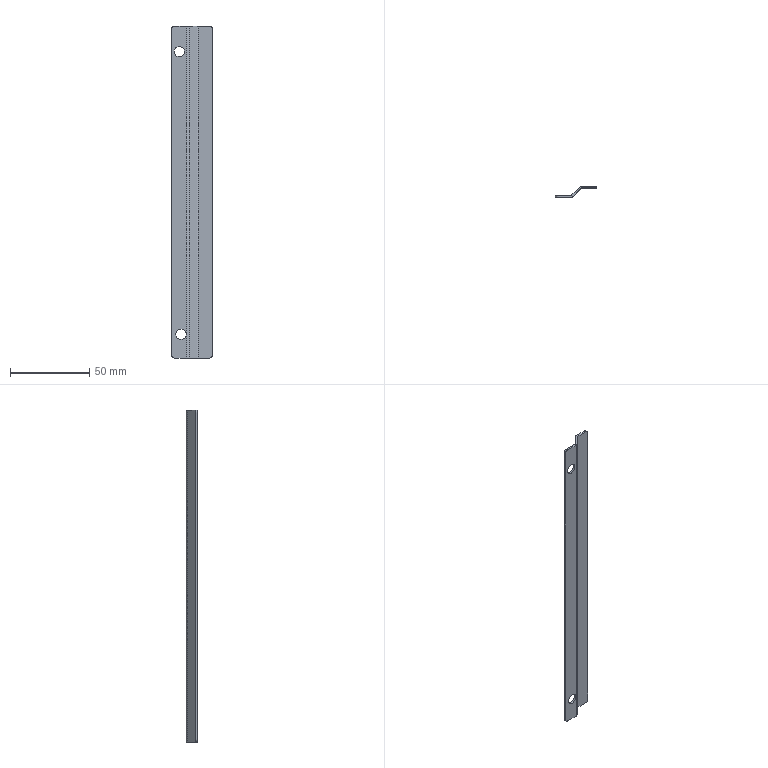Part | SolidWorks | features BreakCorner 1, FlatPattern 1, ICE 1, SMBaseFlange 1, SheetMetal 1 | 1 solid | 30 faces | box 26 x 7.2 x 210 mm | volume 7055 mm3 | plane 18 | cylinder 12 | commonest cylinder face diameters 4 x4 6.5 x4 2.4 x2 4.8 x2
STEP:
#1=CARTESIAN_POINT('',(6.,-1.2,11.75));
#2=VERTEX_POINT('',#1);
#3=CARTESIAN_POINT('',(6.,-1.2,18.25));
#4=VERTEX_POINT('',#3);
#5=CARTESIAN_POINT('',(6.,-1.2,15.));
#6=DIRECTION('',(0.,1.,0.));
#7=DIRECTION('',(0.,0.,1.));
#8=AXIS2_PLACEMENT_3D('',#5,#6,#7);
#9=CIRCLE('',#8,3.25);
#10=EDGE_CURVE('',#2,#4,#9,.T.);
#11=ORIENTED_EDGE('',*,*,#10,.F.);
#12=CARTESIAN_POINT('',(6.,0.,11.75));
#13=VERTEX_POINT('',#12);
#14=CARTESIAN_POINT('',(6.,-10.,11.75));
#15=DIRECTION('',(0.,1.,0.));
#16=VECTOR('',#15,1000.);
#17=LINE('',#14,#16);
#18=EDGE_CURVE('',#2,#13,#17,.T.);
#19=ORIENTED_EDGE('',*,*,#18,.T.);
#20=CARTESIAN_POINT('',(6.,0.,18.25));
#21=VERTEX_POINT('',#20);
#22=CARTESIAN_POINT('',(6.,0.,15.));
#23=DIRECTION('',(0.,1.,0.));
#24=DIRECTION('',(0.,0.,1.));
#25=AXIS2_PLACEMENT_3D('',#22,#23,#24);
#26=CIRCLE('',#25,3.25);
#27=EDGE_CURVE('',#13,#21,#26,.T.);
#28=ORIENTED_EDGE('',*,*,#27,.T.);
#29=CARTESIAN_POINT('',(6.,-10.,18.25));
#30=DIRECTION('',(0.,1.,0.));
#31=VECTOR('',#30,1000.);
#32=LINE('',#29,#31);
#33=EDGE_CURVE('',#4,#21,#32,.T.);
#34=ORIENTED_EDGE('',*,*,#33,.F.);
#35=EDGE_LOOP('',(#11,#19,#28,#34));
#36=FACE_OUTER_BOUND('',#35,.T.);
#37=CARTESIAN_POINT('',(6.,-10.,15.));
#38=DIRECTION('',(0.,1.,0.));
#39=DIRECTION('',(0.,0.,1.));
#40=AXIS2_PLACEMENT_3D('',#37,#38,#39);
#41=CYLINDRICAL_SURFACE('',#40,3.25);
#42=ADVANCED_FACE('',(#36),#41,.F.);
#43=CARTESIAN_POINT('',(5.,-1.2,190.542));
#44=VERTEX_POINT('',#43);
#45=CARTESIAN_POINT('',(5.,-1.2,197.042));
#46=VERTEX_POINT('',#45);
#47=CARTESIAN_POINT('',(5.,-1.2,193.792));
#48=DIRECTION('',(0.,1.,0.));
#49=DIRECTION('',(0.,0.,1.));
#50=AXIS2_PLACEMENT_3D('',#47,#48,#49);
#51=CIRCLE('',#50,3.25);
#52=EDGE_CURVE('',#44,#46,#51,.T.);
#53=ORIENTED_EDGE('',*,*,#52,.F.);
#54=CARTESIAN_POINT('',(5.,0.,190.542));
#55=VERTEX_POINT('',#54);
#56=CARTESIAN_POINT('',(5.,-10.,190.542));
#57=DIRECTION('',(0.,1.,0.));
#58=VECTOR('',#57,1000.);
#59=LINE('',#56,#58);
#60=EDGE_CURVE('',#44,#55,#59,.T.);
#61=ORIENTED_EDGE('',*,*,#60,.T.);
#62=CARTESIAN_POINT('',(5.,0.,197.042));
#63=VERTEX_POINT('',#62);
#64=CARTESIAN_POINT('',(5.,0.,193.792));
#65=DIRECTION('',(0.,1.,0.));
#66=DIRECTION('',(0.,0.,1.));
#67=AXIS2_PLACEMENT_3D('',#64,#65,#66);
#68=CIRCLE('',#67,3.25);
#69=EDGE_CURVE('',#55,#63,#68,.T.);
#70=ORIENTED_EDGE('',*,*,#69,.T.);
#71=CARTESIAN_POINT('',(5.,-10.,197.042));
#72=DIRECTION('',(0.,1.,0.));
#73=VECTOR('',#72,1000.);
#74=LINE('',#71,#73);
#75=EDGE_CURVE('',#46,#63,#74,.T.);
#76=ORIENTED_EDGE('',*,*,#75,.F.);
#77=EDGE_LOOP('',(#53,#61,#70,#76));
#78=FACE_OUTER_BOUND('',#77,.T.);
#79=CARTESIAN_POINT('',(5.,-10.,193.792));
#80=DIRECTION('',(0.,1.,0.));
#81=DIRECTION('',(0.,0.,1.));
#82=AXIS2_PLACEMENT_3D('',#79,#80,#81);
#83=CYLINDRICAL_SURFACE('',#82,3.25);
#84=ADVANCED_FACE('',(#78),#83,.F.);
#85=CARTESIAN_POINT('',(10.351,0.3515,210.));
#86=VERTEX_POINT('',#85);
#87=CARTESIAN_POINT('',(11.2,-0.4971,210.));
#88=VERTEX_POINT('',#87);
#89=CARTESIAN_POINT('',(10.351,0.3515,210.));
#90=DIRECTION('',(0.7071,-0.7071,0.));
#91=VECTOR('',#90,1000.);
#92=LINE('',#89,#91);
#93=EDGE_CURVE('',#86,#88,#92,.T.);
#94=ORIENTED_EDGE('',*,*,#93,.F.);
#95=CARTESIAN_POINT('',(9.503,0.,210.));
#96=VERTEX_POINT('',#95);
#97=CARTESIAN_POINT('',(9.503,1.2,210.));
#98=DIRECTION('',(0.,0.,1.));
#99=DIRECTION('',(-1.,0.,0.));
#100=AXIS2_PLACEMENT_3D('',#97,#98,#99);
#101=CIRCLE('',#100,1.2);
#102=EDGE_CURVE('',#96,#86,#101,.T.);
#103=ORIENTED_EDGE('',*,*,#102,.F.);
#104=CARTESIAN_POINT('',(9.503,-1.2,210.));
#105=VERTEX_POINT('',#104);
#106=CARTESIAN_POINT('',(9.503,-1.2,210.));
#107=DIRECTION('',(0.,1.,0.));
#108=VECTOR('',#107,1000.);
#109=LINE('',#106,#108);
#110=EDGE_CURVE('',#105,#96,#109,.T.);
#111=ORIENTED_EDGE('',*,*,#110,.F.);
#112=CARTESIAN_POINT('',(9.503,1.2,210.));
#113=DIRECTION('',(0.,0.,1.));
#114=DIRECTION('',(1.,0.,0.));
#115=AXIS2_PLACEMENT_3D('',#112,#113,#114);
#116=CIRCLE('',#115,2.4);
#117=EDGE_CURVE('',#105,#88,#116,.T.);
#118=ORIENTED_EDGE('',*,*,#117,.T.);
#119=EDGE_LOOP('',(#94,#103,#111,#118));
#120=FACE_OUTER_BOUND('',#119,.T.);
#121=CARTESIAN_POINT('',(10.351,0.3515,210.));
#122=DIRECTION('',(0.,0.,1.));
#123=DIRECTION('',(1.,0.,0.));
#124=AXIS2_PLACEMENT_3D('',#121,#122,#123);
#125=PLANE('',#124);
#126=ADVANCED_FACE('',(#120),#125,.T.);
#127=CARTESIAN_POINT('',(15.297,5.297,210.));
#128=VERTEX_POINT('',#127);
#129=CARTESIAN_POINT('',(10.,0.,210.));
#130=DIRECTION('',(0.7071,0.7071,0.));
#131=VECTOR('',#130,1000.);
#132=LINE('',#129,#131);
#133=EDGE_CURVE('',#86,#128,#132,.T.);
#134=ORIENTED_EDGE('',*,*,#133,.F.);
#135=ORIENTED_EDGE('',*,*,#93,.T.);
#136=CARTESIAN_POINT('',(16.146,4.449,210.));
#137=VERTEX_POINT('',#136);
#138=CARTESIAN_POINT('',(10.849,-0.8485,210.));
#139=DIRECTION('',(0.7071,0.7071,0.));
#140=VECTOR('',#139,1000.);
#141=LINE('',#138,#140);
#142=EDGE_CURVE('',#88,#137,#141,.T.);
#143=ORIENTED_EDGE('',*,*,#142,.T.);
#144=CARTESIAN_POINT('',(16.146,4.449,210.));
#145=DIRECTION('',(-0.7071,0.7071,0.));
#146=VECTOR('',#145,1000.);
#147=LINE('',#144,#146);
#148=EDGE_CURVE('',#137,#128,#147,.T.);
#149=ORIENTED_EDGE('',*,*,#148,.T.);
#150=EDGE_LOOP('',(#134,#135,#143,#149));
#151=FACE_OUTER_BOUND('',#150,.T.);
#152=CARTESIAN_POINT('',(9.503,-1.2,210.));
#153=DIRECTION('',(0.,0.,1.));
#154=DIRECTION('',(1.,0.,0.));
#155=AXIS2_PLACEMENT_3D('',#152,#153,#154);
#156=PLANE('',#155);
#157=ADVANCED_FACE('',(#151),#156,.T.);
#158=CARTESIAN_POINT('',(9.503,0.,0.));
#159=VERTEX_POINT('',#158);
#160=CARTESIAN_POINT('',(9.503,-1.2,0.));
#161=VERTEX_POINT('',#160);
#162=CARTESIAN_POINT('',(9.503,0.,0.));
#163=DIRECTION('',(0.,-1.,0.));
#164=VECTOR('',#163,1000.);
#165=LINE('',#162,#164);
#166=EDGE_CURVE('',#159,#161,#165,.T.);
#167=ORIENTED_EDGE('',*,*,#166,.F.);
#168=CARTESIAN_POINT('',(10.351,0.3515,0.));
#169=VERTEX_POINT('',#168);
#170=CARTESIAN_POINT('',(9.503,1.2,0.));
#171=DIRECTION('',(0.,0.,1.));
#172=DIRECTION('',(-1.,0.,0.));
#173=AXIS2_PLACEMENT_3D('',#170,#171,#172);
#174=CIRCLE('',#173,1.2);
#175=EDGE_CURVE('',#159,#169,#174,.T.);
#176=ORIENTED_EDGE('',*,*,#175,.T.);
#177=CARTESIAN_POINT('',(11.2,-0.4971,0.));
#178=VERTEX_POINT('',#177);
#179=CARTESIAN_POINT('',(11.2,-0.4971,0.));
#180=DIRECTION('',(-0.7071,0.7071,0.));
#181=VECTOR('',#180,1000.);
#182=LINE('',#179,#181);
#183=EDGE_CURVE('',#178,#169,#182,.T.);
#184=ORIENTED_EDGE('',*,*,#183,.F.);
#185=CARTESIAN_POINT('',(9.503,1.2,0.));
#186=DIRECTION('',(0.,0.,1.));
#187=DIRECTION('',(1.,0.,0.));
#188=AXIS2_PLACEMENT_3D('',#185,#186,#187);
#189=CIRCLE('',#188,2.4);
#190=EDGE_CURVE('',#161,#178,#189,.T.);
#191=ORIENTED_EDGE('',*,*,#190,.F.);
#192=EDGE_LOOP('',(#167,#176,#184,#191));
#193=FACE_OUTER_BOUND('',#192,.T.);
#194=CARTESIAN_POINT('',(9.503,0.,0.));
#195=DIRECTION('',(0.,0.,-1.));
#196=DIRECTION('',(-1.,0.,0.));
#197=AXIS2_PLACEMENT_3D('',#194,#195,#196);
#198=PLANE('',#197);
#199=ADVANCED_FACE('',(#193),#198,.T.);
#200=CARTESIAN_POINT('',(2.,-1.2,0.));
#201=VERTEX_POINT('',#200);
#202=CARTESIAN_POINT('',(0.,-1.2,0.));
#203=DIRECTION('',(1.,0.,0.));
#204=VECTOR('',#203,1000.);
#205=LINE('',#202,#204);
#206=EDGE_CURVE('',#201,#161,#205,.T.);
#207=ORIENTED_EDGE('',*,*,#206,.F.);
#208=CARTESIAN_POINT('',(2.,0.,0.));
#209=VERTEX_POINT('',#208);
#210=CARTESIAN_POINT('',(2.,-0.4971,0.));
#211=DIRECTION('',(0.,1.,0.));
#212=VECTOR('',#211,1000.);
#213=LINE('',#210,#212);
#214=EDGE_CURVE('',#201,#209,#213,.T.);
#215=ORIENTED_EDGE('',*,*,#214,.T.);
#216=CARTESIAN_POINT('',(0.,0.,0.));
#217=DIRECTION('',(1.,0.,0.));
#218=VECTOR('',#217,1000.);
#219=LINE('',#216,#218);
#220=EDGE_CURVE('',#209,#159,#219,.T.);
#221=ORIENTED_EDGE('',*,*,#220,.T.);
#222=ORIENTED_EDGE('',*,*,#166,.T.);
#223=EDGE_LOOP('',(#207,#215,#221,#222));
#224=FACE_OUTER_BOUND('',#223,.T.);
#225=CARTESIAN_POINT('',(11.2,-0.4971,0.));
#226=DIRECTION('',(0.,0.,-1.));
#227=DIRECTION('',(-1.,0.,0.));
#228=AXIS2_PLACEMENT_3D('',#225,#226,#227);
#229=PLANE('',#228);
#230=ADVANCED_FACE('',(#224),#229,.T.);
#231=CARTESIAN_POINT('',(16.994,6.,210.));
#232=VERTEX_POINT('',#231);
#233=CARTESIAN_POINT('',(16.994,4.8,210.));
#234=VERTEX_POINT('',#233);
#235=CARTESIAN_POINT('',(16.994,6.,210.));
#236=DIRECTION('',(0.,-1.,0.));
#237=VECTOR('',#236,1000.);
#238=LINE('',#235,#237);
#239=EDGE_CURVE('',#232,#234,#238,.T.);
#240=ORIENTED_EDGE('',*,*,#239,.F.);
#241=CARTESIAN_POINT('',(16.994,3.6,210.));
#242=DIRECTION('',(0.,0.,-1.));
#243=DIRECTION('',(1.,0.,0.));
#244=AXIS2_PLACEMENT_3D('',#241,#242,#243);
#245=CIRCLE('',#244,2.4);
#246=EDGE_CURVE('',#128,#232,#245,.T.);
#247=ORIENTED_EDGE('',*,*,#246,.F.);
#248=ORIENTED_EDGE('',*,*,#148,.F.);
#249=CARTESIAN_POINT('',(16.994,3.6,210.));
#250=DIRECTION('',(0.,0.,-1.));
#251=DIRECTION('',(1.,0.,0.));
#252=AXIS2_PLACEMENT_3D('',#249,#250,#251);
#253=CIRCLE('',#252,1.2);
#254=EDGE_CURVE('',#137,#234,#253,.T.);
#255=ORIENTED_EDGE('',*,*,#254,.T.);
#256=EDGE_LOOP('',(#240,#247,#248,#255));
#257=FACE_OUTER_BOUND('',#256,.T.);
#258=CARTESIAN_POINT('',(16.994,6.,210.));
#259=DIRECTION('',(0.,0.,1.));
#260=DIRECTION('',(1.,0.,0.));
#261=AXIS2_PLACEMENT_3D('',#258,#259,#260);
#262=PLANE('',#261);
#263=ADVANCED_FACE('',(#257),#262,.T.);
#264=CARTESIAN_POINT('',(24.,4.8,210.));
#265=VERTEX_POINT('',#264);
#266=CARTESIAN_POINT('',(16.,4.8,210.));
#267=DIRECTION('',(1.,0.,0.));
#268=VECTOR('',#267,1000.);
#269=LINE('',#266,#268);
#270=EDGE_CURVE('',#234,#265,#269,.T.);
#271=ORIENTED_EDGE('',*,*,#270,.T.);
#272=CARTESIAN_POINT('',(24.,6.,210.));
#273=VERTEX_POINT('',#272);
#274=CARTESIAN_POINT('',(24.,4.449,210.));
#275=DIRECTION('',(0.,1.,0.));
#276=VECTOR('',#275,1000.);
#277=LINE('',#274,#276);
#278=EDGE_CURVE('',#265,#273,#277,.T.);
#279=ORIENTED_EDGE('',*,*,#278,.T.);
#280=CARTESIAN_POINT('',(16.,6.,210.));
#281=DIRECTION('',(1.,0.,0.));
#282=VECTOR('',#281,1000.);
#283=LINE('',#280,#282);
#284=EDGE_CURVE('',#232,#273,#283,.T.);
#285=ORIENTED_EDGE('',*,*,#284,.F.);
#286=ORIENTED_EDGE('',*,*,#239,.T.);
#287=EDGE_LOOP('',(#271,#279,#285,#286));
#288=FACE_OUTER_BOUND('',#287,.T.);
#289=CARTESIAN_POINT('',(16.146,4.449,210.));
#290=DIRECTION('',(0.,0.,1.));
#291=DIRECTION('',(1.,0.,0.));
#292=AXIS2_PLACEMENT_3D('',#289,#290,#291);
#293=PLANE('',#292);
#294=ADVANCED_FACE('',(#288),#293,.T.);
#295=CARTESIAN_POINT('',(15.297,5.297,0.));
#296=VERTEX_POINT('',#295);
#297=CARTESIAN_POINT('',(16.146,4.449,0.));
#298=VERTEX_POINT('',#297);
#299=CARTESIAN_POINT('',(15.297,5.297,0.));
#300=DIRECTION('',(0.7071,-0.7071,0.));
#301=VECTOR('',#300,1000.);
#302=LINE('',#299,#301);
#303=EDGE_CURVE('',#296,#298,#302,.T.);
#304=ORIENTED_EDGE('',*,*,#303,.F.);
#305=CARTESIAN_POINT('',(16.994,6.,0.));
#306=VERTEX_POINT('',#305);
#307=CARTESIAN_POINT('',(16.994,3.6,0.));
#308=DIRECTION('',(0.,0.,-1.));
#309=DIRECTION('',(1.,0.,0.));
#310=AXIS2_PLACEMENT_3D('',#307,#308,#309);
#311=CIRCLE('',#310,2.4);
#312=EDGE_CURVE('',#296,#306,#311,.T.);
#313=ORIENTED_EDGE('',*,*,#312,.T.);
#314=CARTESIAN_POINT('',(16.994,4.8,0.));
#315=VERTEX_POINT('',#314);
#316=CARTESIAN_POINT('',(16.994,4.8,0.));
#317=DIRECTION('',(0.,1.,0.));
#318=VECTOR('',#317,1000.);
#319=LINE('',#316,#318);
#320=EDGE_CURVE('',#315,#306,#319,.T.);
#321=ORIENTED_EDGE('',*,*,#320,.F.);
#322=CARTESIAN_POINT('',(16.994,3.6,0.));
#323=DIRECTION('',(0.,0.,-1.));
#324=DIRECTION('',(1.,0.,0.));
#325=AXIS2_PLACEMENT_3D('',#322,#323,#324);
#326=CIRCLE('',#325,1.2);
#327=EDGE_CURVE('',#298,#315,#326,.T.);
#328=ORIENTED_EDGE('',*,*,#327,.F.);
#329=EDGE_LOOP('',(#304,#313,#321,#328));
#330=FACE_OUTER_BOUND('',#329,.T.);
#331=CARTESIAN_POINT('',(15.297,5.297,0.));
#332=DIRECTION('',(0.,0.,-1.));
#333=DIRECTION('',(-1.,0.,0.));
#334=AXIS2_PLACEMENT_3D('',#331,#332,#333);
#335=PLANE('',#334);
#336=ADVANCED_FACE('',(#330),#335,.T.);
#337=CARTESIAN_POINT('',(10.,0.,0.));
#338=DIRECTION('',(0.7071,0.7071,0.));
#339=VECTOR('',#338,1000.);
#340=LINE('',#337,#339);
#341=EDGE_CURVE('',#169,#296,#340,.T.);
#342=ORIENTED_EDGE('',*,*,#341,.T.);
#343=ORIENTED_EDGE('',*,*,#303,.T.);
#344=CARTESIAN_POINT('',(10.849,-0.8485,0.));
#345=DIRECTION('',(0.7071,0.7071,0.));
#346=VECTOR('',#345,1000.);
#347=LINE('',#344,#346);
#348=EDGE_CURVE('',#178,#298,#347,.T.);
#349=ORIENTED_EDGE('',*,*,#348,.F.);
#350=ORIENTED_EDGE('',*,*,#183,.T.);
#351=EDGE_LOOP('',(#342,#343,#349,#350));
#352=FACE_OUTER_BOUND('',#351,.T.);
#353=CARTESIAN_POINT('',(16.994,4.8,0.));
#354=DIRECTION('',(0.,0.,-1.));
#355=DIRECTION('',(-1.,0.,0.));
#356=AXIS2_PLACEMENT_3D('',#353,#354,#355);
#357=PLANE('',#356);
#358=ADVANCED_FACE('',(#352),#357,.T.);
#359=CARTESIAN_POINT('',(26.,4.8,208.));
#360=VERTEX_POINT('',#359);
#361=CARTESIAN_POINT('',(26.,4.8,2.));
#362=VERTEX_POINT('',#361);
#363=CARTESIAN_POINT('',(26.,4.8,210.));
#364=DIRECTION('',(0.,0.,-1.));
#365=VECTOR('',#364,1000.);
#366=LINE('',#363,#365);
#367=EDGE_CURVE('',#360,#362,#366,.T.);
#368=ORIENTED_EDGE('',*,*,#367,.F.);
#369=CARTESIAN_POINT('',(24.,4.8,208.));
#370=DIRECTION('',(0.,-1.,0.));
#371=DIRECTION('',(0.,0.,1.));
#372=AXIS2_PLACEMENT_3D('',#369,#370,#371);
#373=CIRCLE('',#372,2.);
#374=EDGE_CURVE('',#360,#265,#373,.T.);
#375=ORIENTED_EDGE('',*,*,#374,.T.);
#376=ORIENTED_EDGE('',*,*,#270,.F.);
#377=CARTESIAN_POINT('',(16.994,4.8,210.));
#378=DIRECTION('',(0.,0.,-1.));
#379=VECTOR('',#378,1000.);
#380=LINE('',#377,#379);
#381=EDGE_CURVE('',#234,#315,#380,.T.);
#382=ORIENTED_EDGE('',*,*,#381,.T.);
#383=CARTESIAN_POINT('',(24.,4.8,0.));
#384=VERTEX_POINT('',#383);
#385=CARTESIAN_POINT('',(16.,4.8,0.));
#386=DIRECTION('',(1.,0.,0.));
#387=VECTOR('',#386,1000.);
#388=LINE('',#385,#387);
#389=EDGE_CURVE('',#315,#384,#388,.T.);
#390=ORIENTED_EDGE('',*,*,#389,.T.);
#391=CARTESIAN_POINT('',(24.,4.8,2.));
#392=DIRECTION('',(0.,-1.,0.));
#393=DIRECTION('',(0.,0.,1.));
#394=AXIS2_PLACEMENT_3D('',#391,#392,#393);
#395=CIRCLE('',#394,2.);
#396=EDGE_CURVE('',#384,#362,#395,.T.);
#397=ORIENTED_EDGE('',*,*,#396,.T.);
#398=EDGE_LOOP('',(#368,#375,#376,#382,#390,#397));
#399=FACE_OUTER_BOUND('',#398,.T.);
#400=CARTESIAN_POINT('',(16.,4.8,210.));
#401=DIRECTION('',(0.,1.,0.));
#402=DIRECTION('',(0.,0.,1.));
#403=AXIS2_PLACEMENT_3D('',#400,#401,#402);
#404=PLANE('',#403);
#405=ADVANCED_FACE('',(#399),#404,.F.);
#406=CARTESIAN_POINT('',(26.,6.,208.));
#407=VERTEX_POINT('',#406);
#408=CARTESIAN_POINT('',(26.,6.,2.));
#409=VERTEX_POINT('',#408);
#410=CARTESIAN_POINT('',(26.,6.,210.));
#411=DIRECTION('',(0.,0.,-1.));
#412=VECTOR('',#411,1000.);
#413=LINE('',#410,#412);
#414=EDGE_CURVE('',#407,#409,#413,.T.);
#415=ORIENTED_EDGE('',*,*,#414,.F.);
#416=CARTESIAN_POINT('',(26.,6.,208.));
#417=DIRECTION('',(0.,-1.,0.));
#418=VECTOR('',#417,1000.);
#419=LINE('',#416,#418);
#420=EDGE_CURVE('',#407,#360,#419,.T.);
#421=ORIENTED_EDGE('',*,*,#420,.T.);
#422=ORIENTED_EDGE('',*,*,#367,.T.);
#423=CARTESIAN_POINT('',(26.,6.,2.));
#424=DIRECTION('',(0.,1.,0.));
#425=VECTOR('',#424,1000.);
#426=LINE('',#423,#425);
#427=EDGE_CURVE('',#362,#409,#426,.T.);
#428=ORIENTED_EDGE('',*,*,#427,.T.);
#429=EDGE_LOOP('',(#415,#421,#422,#428));
#430=FACE_OUTER_BOUND('',#429,.T.);
#431=CARTESIAN_POINT('',(26.,6.,210.));
#432=DIRECTION('',(1.,0.,0.));
#433=DIRECTION('',(0.,0.,-1.));
#434=AXIS2_PLACEMENT_3D('',#431,#432,#433);
#435=PLANE('',#434);
#436=ADVANCED_FACE('',(#430),#435,.T.);
#437=ORIENTED_EDGE('',*,*,#284,.T.);
#438=CARTESIAN_POINT('',(24.,6.,208.));
#439=DIRECTION('',(0.,1.,0.));
#440=DIRECTION('',(0.,0.,1.));
#441=AXIS2_PLACEMENT_3D('',#438,#439,#440);
#442=CIRCLE('',#441,2.);
#443=EDGE_CURVE('',#273,#407,#442,.T.);
#444=ORIENTED_EDGE('',*,*,#443,.T.);
#445=ORIENTED_EDGE('',*,*,#414,.T.);
#446=CARTESIAN_POINT('',(24.,6.,0.));
#447=VERTEX_POINT('',#446);
#448=CARTESIAN_POINT('',(24.,6.,2.));
#449=DIRECTION('',(0.,1.,0.));
#450=DIRECTION('',(0.,0.,1.));
#451=AXIS2_PLACEMENT_3D('',#448,#449,#450);
#452=CIRCLE('',#451,2.);
#453=EDGE_CURVE('',#409,#447,#452,.T.);
#454=ORIENTED_EDGE('',*,*,#453,.T.);
#455=CARTESIAN_POINT('',(16.,6.,0.));
#456=DIRECTION('',(1.,0.,0.));
#457=VECTOR('',#456,1000.);
#458=LINE('',#455,#457);
#459=EDGE_CURVE('',#306,#447,#458,.T.);
#460=ORIENTED_EDGE('',*,*,#459,.F.);
#461=CARTESIAN_POINT('',(16.994,6.,210.));
#462=DIRECTION('',(0.,0.,-1.));
#463=VECTOR('',#462,1000.);
#464=LINE('',#461,#463);
#465=EDGE_CURVE('',#232,#306,#464,.T.);
#466=ORIENTED_EDGE('',*,*,#465,.F.);
#467=EDGE_LOOP('',(#437,#444,#445,#454,#460,#466));
#468=FACE_OUTER_BOUND('',#467,.T.);
#469=CARTESIAN_POINT('',(16.,6.,210.));
#470=DIRECTION('',(0.,1.,0.));
#471=DIRECTION('',(0.,0.,1.));
#472=AXIS2_PLACEMENT_3D('',#469,#470,#471);
#473=PLANE('',#472);
#474=ADVANCED_FACE('',(#468),#473,.T.);
#475=ORIENTED_EDGE('',*,*,#312,.F.);
#476=CARTESIAN_POINT('',(15.297,5.297,210.));
#477=DIRECTION('',(0.,0.,-1.));
#478=VECTOR('',#477,1000.);
#479=LINE('',#476,#478);
#480=EDGE_CURVE('',#128,#296,#479,.T.);
#481=ORIENTED_EDGE('',*,*,#480,.F.);
#482=ORIENTED_EDGE('',*,*,#246,.T.);
#483=ORIENTED_EDGE('',*,*,#465,.T.);
#484=EDGE_LOOP('',(#475,#481,#482,#483));
#485=FACE_OUTER_BOUND('',#484,.T.);
#486=CARTESIAN_POINT('',(16.994,3.6,210.));
#487=DIRECTION('',(0.,0.,-1.));
#488=DIRECTION('',(-1.,0.,0.));
#489=AXIS2_PLACEMENT_3D('',#486,#487,#488);
#490=CYLINDRICAL_SURFACE('',#489,2.4);
#491=ADVANCED_FACE('',(#485),#490,.T.);
#492=ORIENTED_EDGE('',*,*,#341,.F.);
#493=CARTESIAN_POINT('',(10.351,0.3515,210.));
#494=DIRECTION('',(0.,0.,-1.));
#495=VECTOR('',#494,1000.);
#496=LINE('',#493,#495);
#497=EDGE_CURVE('',#86,#169,#496,.T.);
#498=ORIENTED_EDGE('',*,*,#497,.F.);
#499=ORIENTED_EDGE('',*,*,#133,.T.);
#500=ORIENTED_EDGE('',*,*,#480,.T.);
#501=EDGE_LOOP('',(#492,#498,#499,#500));
#502=FACE_OUTER_BOUND('',#501,.T.);
#503=CARTESIAN_POINT('',(10.,0.,210.));
#504=DIRECTION('',(-0.7071,0.7071,0.));
#505=DIRECTION('',(-0.7071,-0.7071,0.));
#506=AXIS2_PLACEMENT_3D('',#503,#504,#505);
#507=PLANE('',#506);
#508=ADVANCED_FACE('',(#502),#507,.T.);
#509=ORIENTED_EDGE('',*,*,#175,.F.);
#510=CARTESIAN_POINT('',(9.503,0.,210.));
#511=DIRECTION('',(0.,0.,-1.));
#512=VECTOR('',#511,1000.);
#513=LINE('',#510,#512);
#514=EDGE_CURVE('',#96,#159,#513,.T.);
#515=ORIENTED_EDGE('',*,*,#514,.F.);
#516=ORIENTED_EDGE('',*,*,#102,.T.);
#517=ORIENTED_EDGE('',*,*,#497,.T.);
#518=EDGE_LOOP('',(#509,#515,#516,#517));
#519=FACE_OUTER_BOUND('',#518,.T.);
#520=CARTESIAN_POINT('',(9.503,1.2,210.));
#521=DIRECTION('',(0.,0.,-1.));
#522=DIRECTION('',(-1.,0.,0.));
#523=AXIS2_PLACEMENT_3D('',#520,#521,#522);
#524=CYLINDRICAL_SURFACE('',#523,1.2);
#525=ADVANCED_FACE('',(#519),#524,.F.);
#526=CARTESIAN_POINT('',(6.,0.,15.));
#527=DIRECTION('',(0.,1.,0.));
#528=DIRECTION('',(0.,0.,1.));
#529=AXIS2_PLACEMENT_3D('',#526,#527,#528);
#530=CIRCLE('',#529,3.25);
#531=EDGE_CURVE('',#21,#13,#530,.T.);
#532=ORIENTED_EDGE('',*,*,#531,.F.);
#533=ORIENTED_EDGE('',*,*,#27,.F.);
#534=EDGE_LOOP('',(#532,#533));
#535=FACE_BOUND('',#534,.T.);
#536=CARTESIAN_POINT('',(5.,0.,193.792));
#537=DIRECTION('',(0.,1.,0.));
#538=DIRECTION('',(0.,0.,1.));
#539=AXIS2_PLACEMENT_3D('',#536,#537,#538);
#540=CIRCLE('',#539,3.25);
#541=EDGE_CURVE('',#63,#55,#540,.T.);
#542=ORIENTED_EDGE('',*,*,#541,.F.);
#543=ORIENTED_EDGE('',*,*,#69,.F.);
#544=EDGE_LOOP('',(#542,#543));
#545=FACE_BOUND('',#544,.T.);
#546=CARTESIAN_POINT('',(0.,0.,208.));
#547=VERTEX_POINT('',#546);
#548=CARTESIAN_POINT('',(0.,0.,2.));
#549=VERTEX_POINT('',#548);
#550=CARTESIAN_POINT('',(0.,0.,210.));
#551=DIRECTION('',(0.,0.,-1.));
#552=VECTOR('',#551,1000.);
#553=LINE('',#550,#552);
#554=EDGE_CURVE('',#547,#549,#553,.T.);
#555=ORIENTED_EDGE('',*,*,#554,.F.);
#556=CARTESIAN_POINT('',(2.,0.,210.));
#557=VERTEX_POINT('',#556);
#558=CARTESIAN_POINT('',(2.,0.,208.));
#559=DIRECTION('',(0.,1.,0.));
#560=DIRECTION('',(0.,0.,1.));
#561=AXIS2_PLACEMENT_3D('',#558,#559,#560);
#562=CIRCLE('',#561,2.);
#563=EDGE_CURVE('',#547,#557,#562,.T.);
#564=ORIENTED_EDGE('',*,*,#563,.T.);
#565=CARTESIAN_POINT('',(0.,0.,210.));
#566=DIRECTION('',(1.,0.,0.));
#567=VECTOR('',#566,1000.);
#568=LINE('',#565,#567);
#569=EDGE_CURVE('',#557,#96,#568,.T.);
#570=ORIENTED_EDGE('',*,*,#569,.T.);
#571=ORIENTED_EDGE('',*,*,#514,.T.);
#572=ORIENTED_EDGE('',*,*,#220,.F.);
#573=CARTESIAN_POINT('',(2.,0.,2.));
#574=DIRECTION('',(0.,1.,0.));
#575=DIRECTION('',(0.,0.,1.));
#576=AXIS2_PLACEMENT_3D('',#573,#574,#575);
#577=CIRCLE('',#576,2.);
#578=EDGE_CURVE('',#209,#549,#577,.T.);
#579=ORIENTED_EDGE('',*,*,#578,.T.);
#580=EDGE_LOOP('',(#555,#564,#570,#571,#572,#579));
#581=FACE_OUTER_BOUND('',#580,.T.);
#582=CARTESIAN_POINT('',(0.,0.,210.));
#583=DIRECTION('',(0.,1.,0.));
#584=DIRECTION('',(0.,0.,1.));
#585=AXIS2_PLACEMENT_3D('',#582,#583,#584);
#586=PLANE('',#585);
#587=ADVANCED_FACE('',(#535,#545,#581),#586,.T.);
#588=CARTESIAN_POINT('',(0.,-1.2,208.));
#589=VERTEX_POINT('',#588);
#590=CARTESIAN_POINT('',(0.,-1.2,2.));
#591=VERTEX_POINT('',#590);
#592=CARTESIAN_POINT('',(0.,-1.2,210.));
#593=DIRECTION('',(0.,0.,-1.));
#594=VECTOR('',#593,1000.);
#595=LINE('',#592,#594);
#596=EDGE_CURVE('',#589,#591,#595,.T.);
#597=ORIENTED_EDGE('',*,*,#596,.F.);
#598=CARTESIAN_POINT('',(0.,-1.2,208.));
#599=DIRECTION('',(0.,1.,0.));
#600=VECTOR('',#599,1000.);
#601=LINE('',#598,#600);
#602=EDGE_CURVE('',#589,#547,#601,.T.);
#603=ORIENTED_EDGE('',*,*,#602,.T.);
#604=ORIENTED_EDGE('',*,*,#554,.T.);
#605=CARTESIAN_POINT('',(0.,-1.2,2.));
#606=DIRECTION('',(0.,-1.,0.));
#607=VECTOR('',#606,1000.);
#608=LINE('',#605,#607);
#609=EDGE_CURVE('',#549,#591,#608,.T.);
#610=ORIENTED_EDGE('',*,*,#609,.T.);
#611=EDGE_LOOP('',(#597,#603,#604,#610));
#612=FACE_OUTER_BOUND('',#611,.T.);
#613=CARTESIAN_POINT('',(0.,-1.2,210.));
#614=DIRECTION('',(-1.,0.,0.));
#615=DIRECTION('',(0.,0.,1.));
#616=AXIS2_PLACEMENT_3D('',#613,#614,#615);
#617=PLANE('',#616);
#618=ADVANCED_FACE('',(#612),#617,.T.);
#619=CARTESIAN_POINT('',(6.,-1.2,15.));
#620=DIRECTION('',(0.,1.,0.));
#621=DIRECTION('',(0.,0.,1.));
#622=AXIS2_PLACEMENT_3D('',#619,#620,#621);
#623=CIRCLE('',#622,3.25);
#624=EDGE_CURVE('',#4,#2,#623,.T.);
#625=ORIENTED_EDGE('',*,*,#624,.T.);
#626=ORIENTED_EDGE('',*,*,#10,.T.);
#627=EDGE_LOOP('',(#625,#626));
#628=FACE_BOUND('',#627,.T.);
#629=CARTESIAN_POINT('',(5.,-1.2,193.792));
#630=DIRECTION('',(0.,1.,0.));
#631=DIRECTION('',(0.,0.,1.));
#632=AXIS2_PLACEMENT_3D('',#629,#630,#631);
#633=CIRCLE('',#632,3.25);
#634=EDGE_CURVE('',#46,#44,#633,.T.);
#635=ORIENTED_EDGE('',*,*,#634,.T.);
#636=ORIENTED_EDGE('',*,*,#52,.T.);
#637=EDGE_LOOP('',(#635,#636));
#638=FACE_BOUND('',#637,.T.);
#639=CARTESIAN_POINT('',(2.,-1.2,210.));
#640=VERTEX_POINT('',#639);
#641=CARTESIAN_POINT('',(0.,-1.2,210.));
#642=DIRECTION('',(1.,0.,0.));
#643=VECTOR('',#642,1000.);
#644=LINE('',#641,#643);
#645=EDGE_CURVE('',#640,#105,#644,.T.);
#646=ORIENTED_EDGE('',*,*,#645,.F.);
#647=CARTESIAN_POINT('',(2.,-1.2,208.));
#648=DIRECTION('',(0.,-1.,0.));
#649=DIRECTION('',(0.,0.,1.));
#650=AXIS2_PLACEMENT_3D('',#647,#648,#649);
#651=CIRCLE('',#650,2.);
#652=EDGE_CURVE('',#640,#589,#651,.T.);
#653=ORIENTED_EDGE('',*,*,#652,.T.);
#654=ORIENTED_EDGE('',*,*,#596,.T.);
#655=CARTESIAN_POINT('',(2.,-1.2,2.));
#656=DIRECTION('',(0.,-1.,0.));
#657=DIRECTION('',(0.,0.,1.));
#658=AXIS2_PLACEMENT_3D('',#655,#656,#657);
#659=CIRCLE('',#658,2.);
#660=EDGE_CURVE('',#591,#201,#659,.T.);
#661=ORIENTED_EDGE('',*,*,#660,.T.);
#662=ORIENTED_EDGE('',*,*,#206,.T.);
#663=CARTESIAN_POINT('',(9.503,-1.2,210.));
#664=DIRECTION('',(0.,0.,-1.));
#665=VECTOR('',#664,1000.);
#666=LINE('',#663,#665);
#667=EDGE_CURVE('',#105,#161,#666,.T.);
#668=ORIENTED_EDGE('',*,*,#667,.F.);
#669=EDGE_LOOP('',(#646,#653,#654,#661,#662,#668));
#670=FACE_OUTER_BOUND('',#669,.T.);
#671=CARTESIAN_POINT('',(0.,-1.2,210.));
#672=DIRECTION('',(0.,1.,0.));
#673=DIRECTION('',(0.,0.,1.));
#674=AXIS2_PLACEMENT_3D('',#671,#672,#673);
#675=PLANE('',#674);
#676=ADVANCED_FACE('',(#628,#638,#670),#675,.F.);
#677=ORIENTED_EDGE('',*,*,#190,.T.);
#678=CARTESIAN_POINT('',(11.2,-0.4971,210.));
#679=DIRECTION('',(0.,0.,-1.));
#680=VECTOR('',#679,1000.);
#681=LINE('',#678,#680);
#682=EDGE_CURVE('',#88,#178,#681,.T.);
#683=ORIENTED_EDGE('',*,*,#682,.F.);
#684=ORIENTED_EDGE('',*,*,#117,.F.);
#685=ORIENTED_EDGE('',*,*,#667,.T.);
#686=EDGE_LOOP('',(#677,#683,#684,#685));
#687=FACE_OUTER_BOUND('',#686,.T.);
#688=CARTESIAN_POINT('',(9.503,1.2,210.));
#689=DIRECTION('',(0.,0.,-1.));
#690=DIRECTION('',(-1.,0.,0.));
#691=AXIS2_PLACEMENT_3D('',#688,#689,#690);
#692=CYLINDRICAL_SURFACE('',#691,2.4);
#693=ADVANCED_FACE('',(#687),#692,.T.);
#694=ORIENTED_EDGE('',*,*,#348,.T.);
#695=CARTESIAN_POINT('',(16.146,4.449,210.));
#696=DIRECTION('',(0.,0.,-1.));
#697=VECTOR('',#696,1000.);
#698=LINE('',#695,#697);
#699=EDGE_CURVE('',#137,#298,#698,.T.);
#700=ORIENTED_EDGE('',*,*,#699,.F.);
#701=ORIENTED_EDGE('',*,*,#142,.F.);
#702=ORIENTED_EDGE('',*,*,#682,.T.);
#703=EDGE_LOOP('',(#694,#700,#701,#702));
#704=FACE_OUTER_BOUND('',#703,.T.);
#705=CARTESIAN_POINT('',(10.849,-0.8485,210.));
#706=DIRECTION('',(-0.7071,0.7071,0.));
#707=DIRECTION('',(-0.7071,-0.7071,0.));
#708=AXIS2_PLACEMENT_3D('',#705,#706,#707);
#709=PLANE('',#708);
#710=ADVANCED_FACE('',(#704),#709,.F.);
#711=ORIENTED_EDGE('',*,*,#327,.T.);
#712=ORIENTED_EDGE('',*,*,#381,.F.);
#713=ORIENTED_EDGE('',*,*,#254,.F.);
#714=ORIENTED_EDGE('',*,*,#699,.T.);
#715=EDGE_LOOP('',(#711,#712,#713,#714));
#716=FACE_OUTER_BOUND('',#715,.T.);
#717=CARTESIAN_POINT('',(16.994,3.6,210.));
#718=DIRECTION('',(0.,0.,-1.));
#719=DIRECTION('',(-1.,0.,0.));
#720=AXIS2_PLACEMENT_3D('',#717,#718,#719);
#721=CYLINDRICAL_SURFACE('',#720,1.2);
#722=ADVANCED_FACE('',(#716),#721,.F.);
#723=ORIENTED_EDGE('',*,*,#569,.F.);
#724=CARTESIAN_POINT('',(2.,3.6,210.));
#725=DIRECTION('',(0.,-1.,0.));
#726=VECTOR('',#725,1000.);
#727=LINE('',#724,#726);
#728=EDGE_CURVE('',#557,#640,#727,.T.);
#729=ORIENTED_EDGE('',*,*,#728,.T.);
#730=ORIENTED_EDGE('',*,*,#645,.T.);
#731=ORIENTED_EDGE('',*,*,#110,.T.);
#732=EDGE_LOOP('',(#723,#729,#730,#731));
#733=FACE_OUTER_BOUND('',#732,.T.);
#734=CARTESIAN_POINT('',(16.994,3.6,210.));
#735=DIRECTION('',(0.,0.,1.));
#736=DIRECTION('',(1.,0.,0.));
#737=AXIS2_PLACEMENT_3D('',#734,#735,#736);
#738=PLANE('',#737);
#739=ADVANCED_FACE('',(#733),#738,.T.);
#740=ORIENTED_EDGE('',*,*,#459,.T.);
#741=CARTESIAN_POINT('',(24.,4.8,0.));
#742=DIRECTION('',(0.,-1.,0.));
#743=VECTOR('',#742,1000.);
#744=LINE('',#741,#743);
#745=EDGE_CURVE('',#447,#384,#744,.T.);
#746=ORIENTED_EDGE('',*,*,#745,.T.);
#747=ORIENTED_EDGE('',*,*,#389,.F.);
#748=ORIENTED_EDGE('',*,*,#320,.T.);
#749=EDGE_LOOP('',(#740,#746,#747,#748));
#750=FACE_OUTER_BOUND('',#749,.T.);
#751=CARTESIAN_POINT('',(16.994,3.6,0.));
#752=DIRECTION('',(0.,0.,1.));
#753=DIRECTION('',(1.,0.,0.));
#754=AXIS2_PLACEMENT_3D('',#751,#752,#753);
#755=PLANE('',#754);
#756=ADVANCED_FACE('',(#750),#755,.F.);
#757=ORIENTED_EDGE('',*,*,#652,.F.);
#758=ORIENTED_EDGE('',*,*,#728,.F.);
#759=ORIENTED_EDGE('',*,*,#563,.F.);
#760=ORIENTED_EDGE('',*,*,#602,.F.);
#761=EDGE_LOOP('',(#757,#758,#759,#760));
#762=FACE_OUTER_BOUND('',#761,.T.);
#763=CARTESIAN_POINT('',(2.,-1.2,208.));
#764=DIRECTION('',(0.,1.,0.));
#765=DIRECTION('',(0.,0.,1.));
#766=AXIS2_PLACEMENT_3D('',#763,#764,#765);
#767=CYLINDRICAL_SURFACE('',#766,2.);
#768=ADVANCED_FACE('',(#762),#767,.T.);
#769=ORIENTED_EDGE('',*,*,#660,.F.);
#770=ORIENTED_EDGE('',*,*,#609,.F.);
#771=ORIENTED_EDGE('',*,*,#578,.F.);
#772=ORIENTED_EDGE('',*,*,#214,.F.);
#773=EDGE_LOOP('',(#769,#770,#771,#772));
#774=FACE_OUTER_BOUND('',#773,.T.);
#775=CARTESIAN_POINT('',(2.,-0.4971,2.));
#776=DIRECTION('',(0.,1.,0.));
#777=DIRECTION('',(0.,0.,1.));
#778=AXIS2_PLACEMENT_3D('',#775,#776,#777);
#779=CYLINDRICAL_SURFACE('',#778,2.);
#780=ADVANCED_FACE('',(#774),#779,.T.);
#781=ORIENTED_EDGE('',*,*,#443,.F.);
#782=ORIENTED_EDGE('',*,*,#278,.F.);
#783=ORIENTED_EDGE('',*,*,#374,.F.);
#784=ORIENTED_EDGE('',*,*,#420,.F.);
#785=EDGE_LOOP('',(#781,#782,#783,#784));
#786=FACE_OUTER_BOUND('',#785,.T.);
#787=CARTESIAN_POINT('',(24.,6.,208.));
#788=DIRECTION('',(0.,-1.,0.));
#789=DIRECTION('',(0.,0.,-1.));
#790=AXIS2_PLACEMENT_3D('',#787,#788,#789);
#791=CYLINDRICAL_SURFACE('',#790,2.);
#792=ADVANCED_FACE('',(#786),#791,.T.);
#793=ORIENTED_EDGE('',*,*,#453,.F.);
#794=ORIENTED_EDGE('',*,*,#427,.F.);
#795=ORIENTED_EDGE('',*,*,#396,.F.);
#796=ORIENTED_EDGE('',*,*,#745,.F.);
#797=EDGE_LOOP('',(#793,#794,#795,#796));
#798=FACE_OUTER_BOUND('',#797,.T.);
#799=CARTESIAN_POINT('',(24.,3.6,2.));
#800=DIRECTION('',(0.,1.,0.));
#801=DIRECTION('',(0.,0.,1.));
#802=AXIS2_PLACEMENT_3D('',#799,#800,#801);
#803=CYLINDRICAL_SURFACE('',#802,2.);
#804=ADVANCED_FACE('',(#798),#803,.T.);
#805=ORIENTED_EDGE('',*,*,#60,.F.);
#806=ORIENTED_EDGE('',*,*,#634,.F.);
#807=ORIENTED_EDGE('',*,*,#75,.T.);
#808=ORIENTED_EDGE('',*,*,#541,.T.);
#809=EDGE_LOOP('',(#805,#806,#807,#808));
#810=FACE_OUTER_BOUND('',#809,.T.);
#811=CARTESIAN_POINT('',(5.,-10.,193.792));
#812=DIRECTION('',(0.,1.,0.));
#813=DIRECTION('',(0.,0.,1.));
#814=AXIS2_PLACEMENT_3D('',#811,#812,#813);
#815=CYLINDRICAL_SURFACE('',#814,3.25);
#816=ADVANCED_FACE('',(#810),#815,.F.);
#817=ORIENTED_EDGE('',*,*,#18,.F.);
#818=ORIENTED_EDGE('',*,*,#624,.F.);
#819=ORIENTED_EDGE('',*,*,#33,.T.);
#820=ORIENTED_EDGE('',*,*,#531,.T.);
#821=EDGE_LOOP('',(#817,#818,#819,#820));
#822=FACE_OUTER_BOUND('',#821,.T.);
#823=CARTESIAN_POINT('',(6.,-10.,15.));
#824=DIRECTION('',(0.,1.,0.));
#825=DIRECTION('',(0.,0.,1.));
#826=AXIS2_PLACEMENT_3D('',#823,#824,#825);
#827=CYLINDRICAL_SURFACE('',#826,3.25);
#828=ADVANCED_FACE('',(#822),#827,.F.);
#829=CLOSED_SHELL('',(#42,#84,#126,#157,#199,#230,#263,#294,#336,#358,#405,#436,#474,#491,#508,#525,#587,#618,#676,#693,#710,#722,#739,#756,#768,#780,#792,#804,#816,#828));
#830=MANIFOLD_SOLID_BREP('',#829);
#831=CARTESIAN_POINT('',(0.,0.,0.));
#832=DIRECTION('',(0.,0.,1.));
#833=DIRECTION('',(1.,0.,0.));
#834=AXIS2_PLACEMENT_3D('',#831,#832,#833);
#835=(LENGTH_UNIT()NAMED_UNIT(*)SI_UNIT(.MILLI.,.METRE.));
#836=UNCERTAINTY_MEASURE_WITH_UNIT(LENGTH_MEASURE(0.00001),#835,'','');
#837=(NAMED_UNIT(*)PLANE_ANGLE_UNIT()SI_UNIT($,.RADIAN.));
#838=(NAMED_UNIT(*)SI_UNIT($,.STERADIAN.)SOLID_ANGLE_UNIT());
#839=(GEOMETRIC_REPRESENTATION_CONTEXT(3)GLOBAL_UNCERTAINTY_ASSIGNED_CONTEXT((#836))GLOBAL_UNIT_ASSIGNED_CONTEXT((#835,#837,#838))REPRESENTATION_CONTEXT('',''));
#840=ADVANCED_BREP_SHAPE_REPRESENTATION('',(#830,#834),#839);